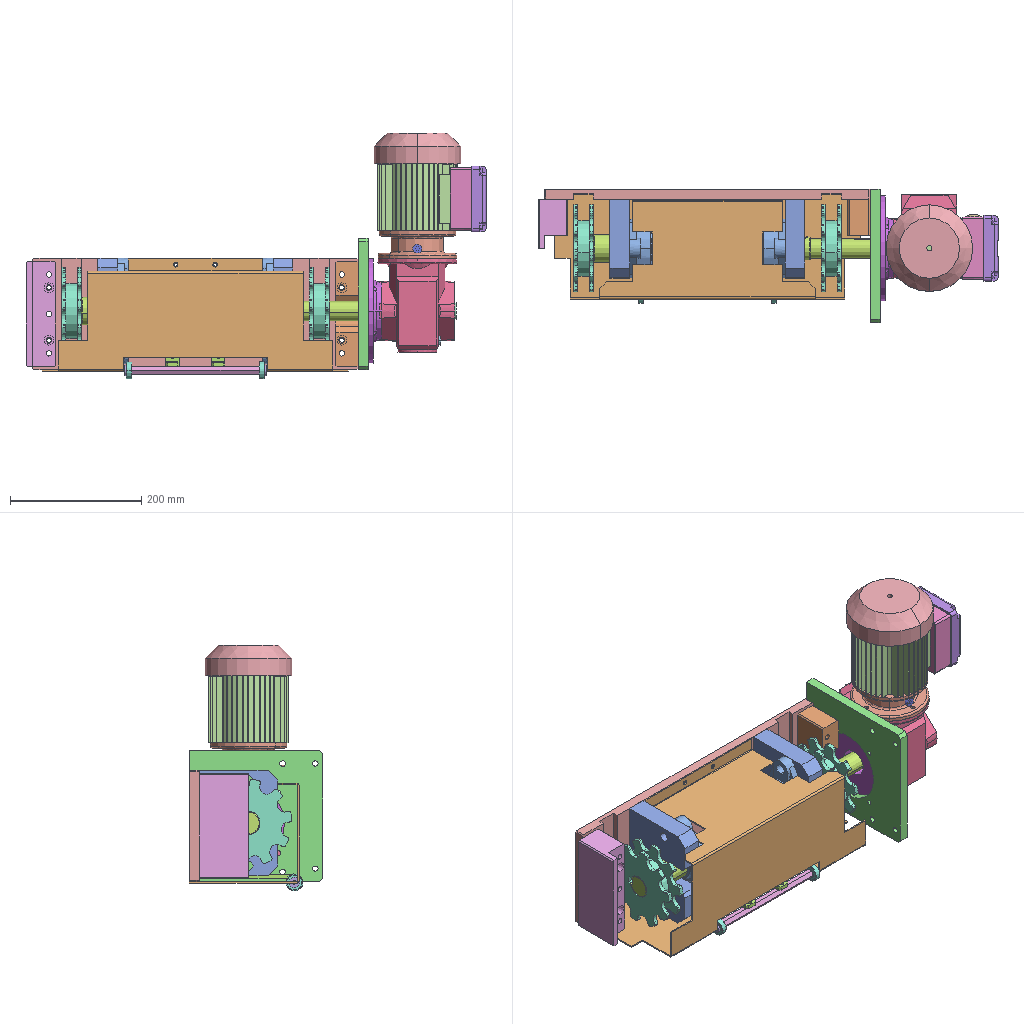Assembly | SolidWorks | 28 different items | 34 placed | box 700 x 203 x 374 mm
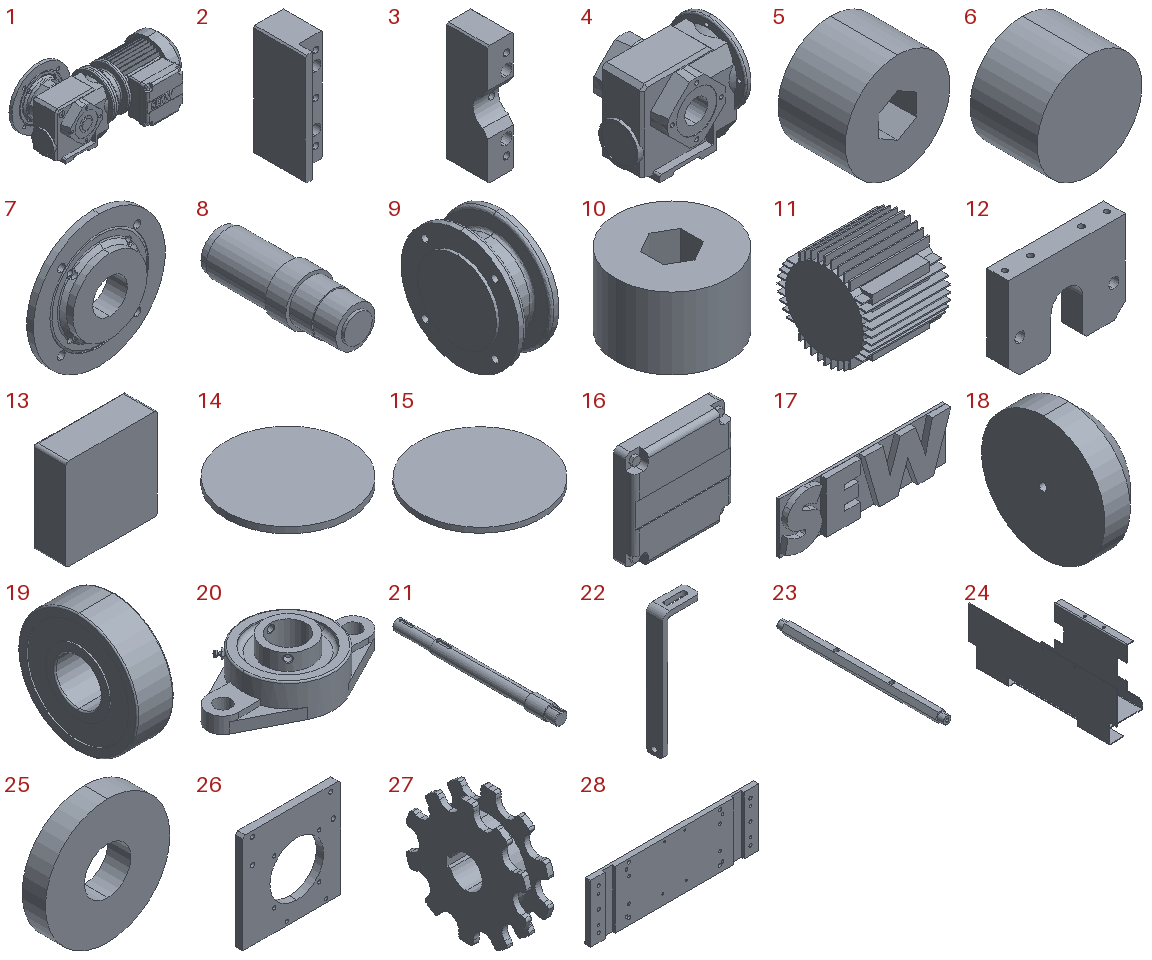Parts list (item | name | quantity | parent item | size | volume | features):
1 | (subassembly) | x1 | - | 351 x 182.5 x 162 mm | 4012734 mm3 | -
2 | - | x1 | - | 44.75 x 75 x 160 mm | 399871 mm3 | features HoleWzd 2, Chamfer 1, Cut 1, Extrusion 1
3 | - | x1 | - | 34 x 55 x 160 mm | 251328 mm3 | features Chamfer 2, HoleWzd 2, Extrusion 1, ICE 1
4 | - | x1 | in 1 | 143 x 120 x 142 mm | 1389830 mm3 | features BaseBody 1
5 | - | x1 | in 1 | 14 x 9 x 14 mm | 1299 mm3 | features BaseBody 1
6 | - | x1 | in 1 | 14 x 9 x 14 mm | 1299 mm3 | features BaseBody 1
7 | - | x1 | in 1 | 160 x 24 x 160 mm | 238568 mm3 | features ICE 3, BaseBody 1, CirPattern 1
8 | - | x1 | in 1 | 43 x 122.5 x 43 mm | 103084 mm3 | features BaseBody 1
9 | - | x1 | in 1 | 45 x 120 x 120 mm | 320577 mm3 | features BaseBody 1
10 | - | x1 | in 1 | 14 x 14 x 9 mm | 1299 mm3 | features BaseBody 1
11 | - | x1 | in 1 | 102 x 122 x 122 mm | 884304 mm3 | features BaseBody 1
12 | - | x2 | - | 161 x 30 x 120 mm | 471064 mm3 | features Chamfer 2, HoleWzd 2, ICE 2, Extrusion 1
13 | - | x1 | in 1 | 95 x 33 x 95 mm | 297490 mm3 | features BaseBody 1
14 | - | x1 | in 1 | 20 x 20 x 3.972 mm | 728.684 mm3 | features BaseBody 1
15 | - | x1 | in 1 | 24 x 24 x 4.478 mm | 1175 mm3 | features BaseBody 1
16 | - | x1 | in 1 | 100 x 21.5 x 100 mm | 204377 mm3 | features BaseBody 1
17 | - | x1 | in 1 | 58.086 x 3 x 18.091 mm | 2435 mm3 | features BaseBody 1
18 | - | x1 | in 1 | 47 x 132 x 132 mm | 566262 mm3 | features BaseBody 1
19 | - | x2 | - | 8 x 26 x 26 mm | 3459 mm3 | features RefAxis 9, 3DProfileFeature 3, Revolution 1
20 | - | x2 | - | 161 x 90 x 44.4 mm | 197699 mm3 | features ICE 5, RevCut 2, Revolution 2
21 | - | x1 | - | 42 x 470 x 42 mm | 443457 mm3 | features ICE 6, Chamfer 2, Extrusion 1
22 | - | x2 | - | 45 x 20 x 151 mm | 21164 mm3 | features ICE 3, Fillet 2, Chamfer 1, Extrusion 1
23 | - | x1 | - | 13.856 x 210 x 12 mm | 24621 mm3 | features HoleWzd 3, ICE 2, Chamfer 1, Extrusion 1
24 | - | x1 | - | 172 x 466 x 167 mm | 311713 mm3 | features ICE 6, Cut 2, Fillet 2, Chamfer 1, Extrusion 1
25 | - | x2 | - | 16 x 3 x 16 mm | 518.363 mm3 | features Extrusion 1
26 | - | x1 | - | 200 x 15 x 203 mm | 456778 mm3 | features HoleWzd 3, ICE 3, Chamfer 1, Cut 1, Extrusion 1
27 | - | x2 | - | 30 x 129.474 x 133 mm | 202077 mm3 | features ICE 3, CirPattern 1, Extrusion 1, Fillet 1, RevCut 1
28 | - | x1 | - | 496 x 15 x 170 mm | 1153313 mm3 | features HoleWzd 7, ICE 2, Chamfer 1, Cut 1, Extrusion 1, MirrorPattern 1
Mates (type | each side: item.copy, entity, surface, feature):
In the top assembly
Coincident | 28.1 face plane Boss-Extrude1 | 22.1 face plane Boss-Extrude1
Coincident | 28.1 face plane Boss-Extrude1 | 22.2 face plane Boss-Extrude1
Concentric | 22.2 face cylinder Cut-Extrude2 | 23.1 face cylinder M6 Tapped Hole1
Concentric | 22.1 face cylinder Cut-Extrude2 | 23.1 face cylinder M6 Tapped Hole1
Coincident | 22.2 face plane Boss-Extrude1 | 23.1 face plane Boss-Extrude1
Coincident | 22.1 face plane Boss-Extrude1 | 23.1 face plane Boss-Extrude1
Concentric | 23.1 face cylinder Cut-Extrude1 | 19.1 face cylinder Revolve1
Coincident | 23.1 face plane Cut-Extrude1 | 19.1 face plane Revolve1
Coincident | 23.1 face plane Cut-Extrude2 | 19.2 face plane Revolve1
Concentric | 23.1 face cylinder Cut-Extrude2 | 19.2 face cylinder Revolve1
DistanceDim | 22.1 face plane Boss-Extrude1 | 28.1 face plane Boss-Extrude1
Coincident | 28.1 face plane Boss-Extrude1 | 24.1 face plane Boss-Extrude1 | 2 times
Concentric | 23.1 face cylinder M5 Tapped Hole2 | 25.1 face cylinder Boss-Extrude1
Coincident | 19.1 face plane Revolve1 | 25.1 face plane Boss-Extrude1
Coincident | 19.2 face plane Revolve1 | 25.2 face plane Boss-Extrude1
Concentric | 23.1 face cylinder M5 Tapped Hole1 | 25.2 face cylinder Boss-Extrude1
Coincident | 28.1 face plane Boss-Extrude1 | 26.1 face plane Boss-Extrude1
Concentric | 28.1 face cylinder M6 Tapped Hole1 | 26.1 face cylinder CBORE for M6 Hex Socket Head Cap Screw1 | 2 times
Coincident | 26.1 face plane Boss-Extrude1 | 7.1 face plane Input1
DistanceDim | 12.1 face plane Boss-Extrude1 | 12.2 face plane Boss-Extrude1
Width | 28.1 face plane Boss-Extrude1 | 28.1 face plane Boss-Extrude1 | 12.2 face plane Boss-Extrude1 | 12.1 face plane Boss-Extrude1
Width | 28.1 face plane Boss-Extrude1 | 28.1 face plane Boss-Extrude1 | 22.1 face plane Boss-Extrude1 | 22.2 face plane Boss-Extrude1
Width | 28.1 face plane Boss-Extrude1 | 28.1 face plane Boss-Extrude1 | 24.1 face plane Boss-Extrude2 | 24.1 face plane Boss-Extrude3
Parallel | 26.1 face plane Boss-Extrude2 | 4.1 face plane Input1
Coincident | 28.1 face plane Boss-Extrude1 | 12.2 face plane Boss-Extrude1
Coincident | 28.1 face plane Boss-Extrude1 | 12.1 face plane Boss-Extrude1 | 2 times
Concentric | 12.1 face cylinder M16 Tapped Hole1 | 20.1 face cylinder Cut-Extrude5
Concentric | 12.1 face cylinder M16 Tapped Hole1 | 20.1 face cylinder Cut-Extrude4
Coincident | 12.1 face plane Boss-Extrude1 | 20.1 face plane Revolve2
Concentric | 27.1 face cylinder Cut-Revolve1 | 21.1 face cylinder Boss-Extrude1
Coincident | 27.1 face plane Boss-Extrude1 | 21.1 face plane Boss-Extrude2
Concentric | 20.1 face cylinder Revolve2 | 21.1 face cylinder Boss-Extrude2
Coincident | 20.1 face plane Revolve2 | 21.1 face plane Boss-Extrude2
Coincident | 28.1 face plane Boss-Extrude1 | 2.1 face plane Boss-Extrude1
Concentric | 28.1 face cylinder CBORE for M8 Hex Socket Head Cap Screw2 | 2.1 face cylinder Ø8.5 (8.5) Diameter Hole1 | 2 times
Coincident | 12.1 face plane Boss-Extrude1 | 12.2 face plane Boss-Extrude1
Concentric | 7.1 face cylinder Input1 | 21.1 face cylinder Boss-Extrude4
Coincident | 26.1 face plane Boss-Extrude1 | 3.1 face plane Boss-Extrude1
Coincident | 28.1 face plane Boss-Extrude1 | 3.1 face plane Boss-Extrude1
Coincident | 2.1 face plane Boss-Extrude1 | 3.1 face plane Boss-Extrude1
Coincident | 27.1 face plane Cut-Extrude2 | 21.1 face plane Cut-Extrude1
In subassembly 1
DistanceDim | 5.1 face plane Input1 | 4.2 face plane Input1 | 2 times
DistanceDim | 5.1 plane | 4.2 face plane Input1
DistanceDim | 6.1 face plane Input1 | 4.2 face plane Input1 | 2 times
DistanceDim | 6.1 plane | 4.2 face plane Input1
Concentric | 7.2 face cylinder Input1 | 8.1 face cone Input1
DistanceDim | 7.2 face plane Input1 | 4.2 face plane Input1
DistanceDim | 7.2 plane | 4.2 face plane Input1
DistanceDim | 8.1 face plane Input1 | 4.2 face plane Input1
DistanceDim | 8.1 plane | 4.2 face plane Input1
Concentric | 4.2 face cylinder Input1 | 9.1 face cylinder Input1 | 2 times
Coincident | 4.2 face plane Input1 | 9.1 face plane Input1
DistanceDim | 10.1 face plane Input1 | 4.2 face plane Input1
DistanceDim | 9.1 face plane Input1 | 10.1 face plane Input1